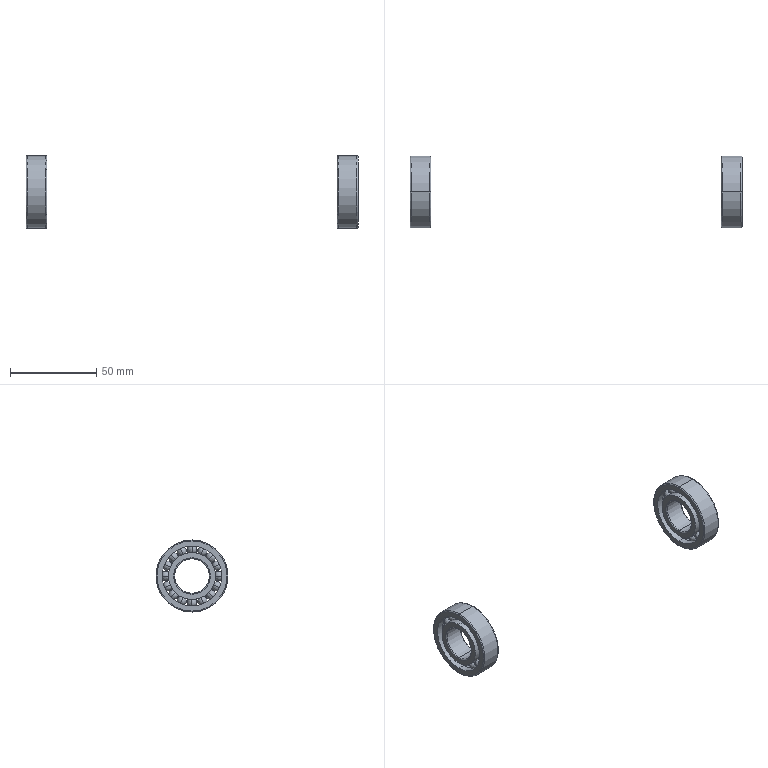Part | NX | features BREP 1 | 2 solids | 272 faces | box 193 x 42 x 42 mm | volume 18872 mm3 | sphere 128 | torus 112 | cylinder 24 | plane 8 | commonest cylinder face diameters 27.333 x8 34.667 x8 20 x4 42 x4